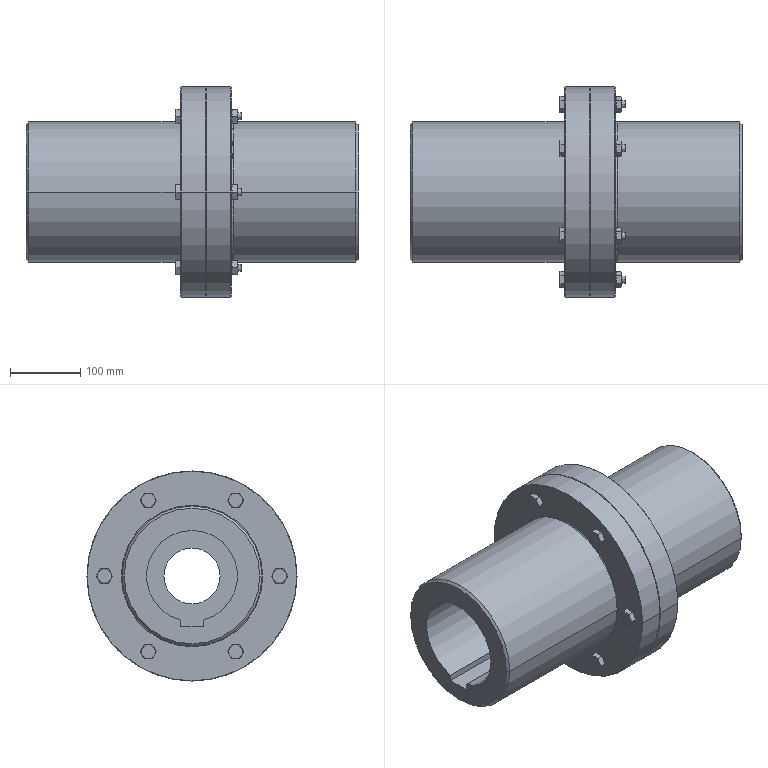Part | SolidWorks | features ICE 15, Chamfer 6, Revolution 3, CirPattern 2, Fillet 2 | 1 solid | 320 faces | box 474 x 300 x 300 mm | volume 12928515 mm3 | cone 144 | plane 111 | cylinder 61 | torus 4 | commonest cylinder face diameters 10 x36 20 x12 200 x4 300 x4 80 x2 210 x2